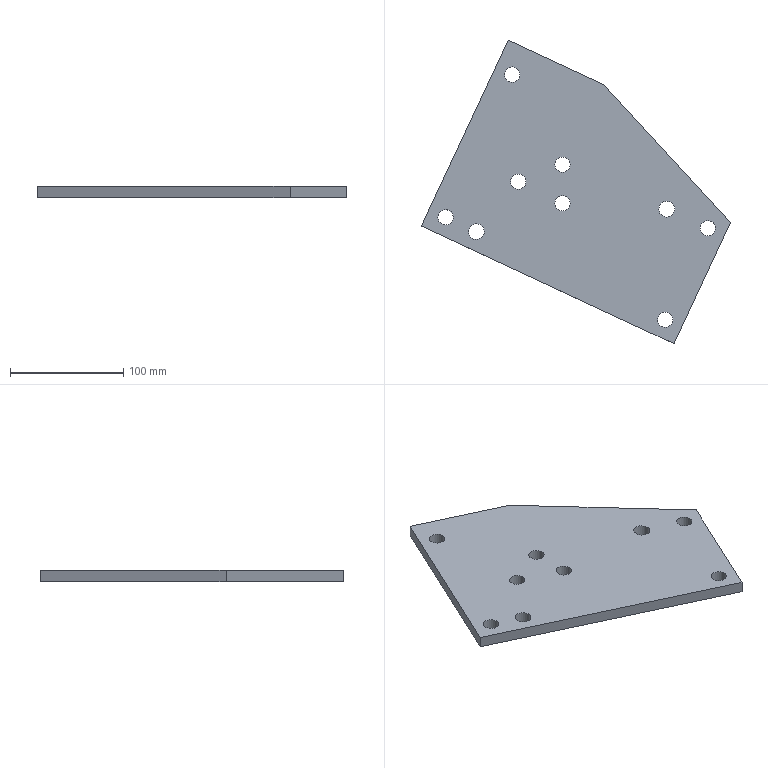Part | NX | features 6 2 | 1 solid | 16 faces | box 272.821 x 268.006 x 10 mm | volume 384202 mm3 | cylinder 9 | plane 7 | commonest cylinder face diameters 13.5 x7 14.001 x2
STEP:
#1=CARTESIAN_POINT('',(505.114,-156.901,101.));
#2=VERTEX_POINT('',#1);
#3=CARTESIAN_POINT('',(455.245,-263.846,101.));
#4=VERTEX_POINT('',#3);
#5=CARTESIAN_POINT('',(485.04,-199.951,101.));
#6=DIRECTION('',(-0.4226,-0.9063,0.));
#7=VECTOR('',#6,1000.);
#8=LINE('',#5,#7);
#9=EDGE_CURVE('',#2,#4,#8,.T.);
#10=ORIENTED_EDGE('',*,*,#9,.F.);
#11=CARTESIAN_POINT('',(393.754,-35.46,101.));
#12=VERTEX_POINT('',#11);
#13=CARTESIAN_POINT('',(202.399,173.217,101.));
#14=DIRECTION('',(-0.6759,0.737,0.));
#15=VECTOR('',#14,1000.);
#16=LINE('',#13,#15);
#17=EDGE_CURVE('',#2,#12,#16,.T.);
#18=ORIENTED_EDGE('',*,*,#17,.T.);
#19=CARTESIAN_POINT('',(308.788,4.16,101.));
#20=VERTEX_POINT('',#19);
#21=CARTESIAN_POINT('',(415.732,-45.709,101.));
#22=DIRECTION('',(0.9063,-0.4226,0.));
#23=VECTOR('',#22,1000.);
#24=LINE('',#21,#23);
#25=EDGE_CURVE('',#20,#12,#24,.T.);
#26=ORIENTED_EDGE('',*,*,#25,.F.);
#27=CARTESIAN_POINT('',(232.294,-159.881,101.));
#28=VERTEX_POINT('',#27);
#29=CARTESIAN_POINT('',(262.088,-95.987,101.));
#30=DIRECTION('',(0.4226,0.9063,0.));
#31=VECTOR('',#30,1000.);
#32=LINE('',#29,#31);
#33=EDGE_CURVE('',#28,#20,#32,.T.);
#34=ORIENTED_EDGE('',*,*,#33,.F.);
#35=CARTESIAN_POINT('',(339.238,-209.75,101.));
#36=DIRECTION('',(-0.9063,0.4226,0.));
#37=VECTOR('',#36,1000.);
#38=LINE('',#35,#37);
#39=EDGE_CURVE('',#4,#28,#38,.T.);
#40=ORIENTED_EDGE('',*,*,#39,.F.);
#41=EDGE_LOOP('',(#10,#18,#26,#34,#40));
#42=FACE_BOUND('',#41,.T.);
#43=CARTESIAN_POINT('',(455.212,-147.975,101.));
#44=VERTEX_POINT('',#43);
#45=CARTESIAN_POINT('',(448.867,-145.017,101.));
#46=DIRECTION('',(0.,0.,-1.));
#47=DIRECTION('',(0.9063,-0.4226,0.));
#48=AXIS2_PLACEMENT_3D('',#45,#46,#47);
#49=CIRCLE('',#48,7.);
#50=EDGE_CURVE('',#44,#44,#49,.T.);
#51=ORIENTED_EDGE('',*,*,#50,.T.);
#52=EDGE_LOOP('',(#51));
#53=FACE_BOUND('',#52,.T.);
#54=CARTESIAN_POINT('',(318.418,-29.018,101.));
#55=VERTEX_POINT('',#54);
#56=CARTESIAN_POINT('',(312.3,-26.166,101.));
#57=DIRECTION('',(0.,0.,-1.));
#58=DIRECTION('',(0.9063,-0.4226,0.));
#59=AXIS2_PLACEMENT_3D('',#56,#57,#58);
#60=CIRCLE('',#59,6.75);
#61=EDGE_CURVE('',#55,#55,#60,.T.);
#62=ORIENTED_EDGE('',*,*,#61,.T.);
#63=EDGE_LOOP('',(#62));
#64=FACE_BOUND('',#63,.T.);
#65=CARTESIAN_POINT('',(491.237,-164.774,101.));
#66=VERTEX_POINT('',#65);
#67=CARTESIAN_POINT('',(485.119,-161.921,101.));
#68=DIRECTION('',(0.,0.,-1.));
#69=DIRECTION('',(0.9063,-0.4226,0.));
#70=AXIS2_PLACEMENT_3D('',#67,#68,#69);
#71=CIRCLE('',#70,6.75);
#72=EDGE_CURVE('',#66,#66,#71,.T.);
#73=ORIENTED_EDGE('',*,*,#72,.T.);
#74=EDGE_LOOP('',(#73));
#75=FACE_BOUND('',#74,.T.);
#76=CARTESIAN_POINT('',(259.674,-154.995,101.));
#77=VERTEX_POINT('',#76);
#78=CARTESIAN_POINT('',(253.556,-152.142,101.));
#79=DIRECTION('',(0.,0.,-1.));
#80=DIRECTION('',(0.9063,-0.4226,0.));
#81=AXIS2_PLACEMENT_3D('',#78,#79,#80);
#82=CIRCLE('',#81,6.75);
#83=EDGE_CURVE('',#77,#77,#82,.T.);
#84=ORIENTED_EDGE('',*,*,#83,.T.);
#85=EDGE_LOOP('',(#84));
#86=FACE_BOUND('',#85,.T.);
#87=CARTESIAN_POINT('',(453.624,-245.435,101.));
#88=VERTEX_POINT('',#87);
#89=CARTESIAN_POINT('',(447.506,-242.583,101.));
#90=DIRECTION('',(0.,0.,-1.));
#91=DIRECTION('',(0.9063,-0.4226,0.));
#92=AXIS2_PLACEMENT_3D('',#89,#90,#91);
#93=CIRCLE('',#92,6.75);
#94=EDGE_CURVE('',#88,#88,#93,.T.);
#95=ORIENTED_EDGE('',*,*,#94,.T.);
#96=EDGE_LOOP('',(#95));
#97=FACE_BOUND('',#96,.T.);
#98=CARTESIAN_POINT('',(287.09,-167.779,101.));
#99=VERTEX_POINT('',#98);
#100=CARTESIAN_POINT('',(280.746,-164.821,101.));
#101=DIRECTION('',(0.,0.,-1.));
#102=DIRECTION('',(0.9063,-0.4226,0.));
#103=AXIS2_PLACEMENT_3D('',#100,#101,#102);
#104=CIRCLE('',#103,7.);
#105=EDGE_CURVE('',#99,#99,#104,.T.);
#106=ORIENTED_EDGE('',*,*,#105,.T.);
#107=EDGE_LOOP('',(#106));
#108=FACE_BOUND('',#107,.T.);
#109=CARTESIAN_POINT('',(363.523,-105.747,101.));
#110=VERTEX_POINT('',#109);
#111=CARTESIAN_POINT('',(356.773,-105.747,101.));
#112=DIRECTION('',(0.,0.,1.));
#113=DIRECTION('',(1.,0.,0.));
#114=AXIS2_PLACEMENT_3D('',#111,#112,#113);
#115=CIRCLE('',#114,6.75);
#116=EDGE_CURVE('',#110,#110,#115,.T.);
#117=ORIENTED_EDGE('',*,*,#116,.F.);
#118=EDGE_LOOP('',(#117));
#119=FACE_BOUND('',#118,.T.);
#120=CARTESIAN_POINT('',(363.523,-139.747,101.));
#121=VERTEX_POINT('',#120);
#122=CARTESIAN_POINT('',(356.773,-139.747,101.));
#123=DIRECTION('',(0.,0.,1.));
#124=DIRECTION('',(1.,0.,0.));
#125=AXIS2_PLACEMENT_3D('',#122,#123,#124);
#126=CIRCLE('',#125,6.75);
#127=EDGE_CURVE('',#121,#121,#126,.T.);
#128=ORIENTED_EDGE('',*,*,#127,.F.);
#129=EDGE_LOOP('',(#128));
#130=FACE_BOUND('',#129,.T.);
#131=CARTESIAN_POINT('',(324.523,-120.747,101.));
#132=VERTEX_POINT('',#131);
#133=CARTESIAN_POINT('',(317.773,-120.747,101.));
#134=DIRECTION('',(0.,0.,1.));
#135=DIRECTION('',(1.,0.,0.));
#136=AXIS2_PLACEMENT_3D('',#133,#134,#135);
#137=CIRCLE('',#136,6.75);
#138=EDGE_CURVE('',#132,#132,#137,.T.);
#139=ORIENTED_EDGE('',*,*,#138,.F.);
#140=EDGE_LOOP('',(#139));
#141=FACE_BOUND('',#140,.T.);
#142=CARTESIAN_POINT('',(239.919,207.622,101.));
#143=DIRECTION('',(0.,0.,1.));
#144=DIRECTION('',(-0.9063,0.4226,0.));
#145=AXIS2_PLACEMENT_3D('',#142,#143,#144);
#146=PLANE('',#145);
#147=ADVANCED_FACE('',(#42,#53,#64,#75,#86,#97,#108,#119,#130,#141),#146,.T.);
#148=CARTESIAN_POINT('',(393.754,-35.46,91.));
#149=VERTEX_POINT('',#148);
#150=CARTESIAN_POINT('',(308.788,4.16,91.));
#151=VERTEX_POINT('',#150);
#152=CARTESIAN_POINT('',(415.732,-45.709,91.));
#153=DIRECTION('',(-0.9063,0.4226,0.));
#154=VECTOR('',#153,1000.);
#155=LINE('',#152,#154);
#156=EDGE_CURVE('',#149,#151,#155,.T.);
#157=ORIENTED_EDGE('',*,*,#156,.F.);
#158=CARTESIAN_POINT('',(505.114,-156.901,91.));
#159=VERTEX_POINT('',#158);
#160=CARTESIAN_POINT('',(437.453,-83.115,91.));
#161=DIRECTION('',(0.6759,-0.737,0.));
#162=VECTOR('',#161,1000.);
#163=LINE('',#160,#162);
#164=EDGE_CURVE('',#149,#159,#163,.T.);
#165=ORIENTED_EDGE('',*,*,#164,.T.);
#166=CARTESIAN_POINT('',(455.245,-263.846,91.));
#167=VERTEX_POINT('',#166);
#168=CARTESIAN_POINT('',(485.04,-199.951,91.));
#169=DIRECTION('',(0.4226,0.9063,0.));
#170=VECTOR('',#169,1000.);
#171=LINE('',#168,#170);
#172=EDGE_CURVE('',#167,#159,#171,.T.);
#173=ORIENTED_EDGE('',*,*,#172,.F.);
#174=CARTESIAN_POINT('',(232.294,-159.881,91.));
#175=VERTEX_POINT('',#174);
#176=CARTESIAN_POINT('',(339.238,-209.75,91.));
#177=DIRECTION('',(0.9063,-0.4226,0.));
#178=VECTOR('',#177,1000.);
#179=LINE('',#176,#178);
#180=EDGE_CURVE('',#175,#167,#179,.T.);
#181=ORIENTED_EDGE('',*,*,#180,.F.);
#182=CARTESIAN_POINT('',(262.088,-95.987,91.));
#183=DIRECTION('',(-0.4226,-0.9063,0.));
#184=VECTOR('',#183,1000.);
#185=LINE('',#182,#184);
#186=EDGE_CURVE('',#151,#175,#185,.T.);
#187=ORIENTED_EDGE('',*,*,#186,.F.);
#188=EDGE_LOOP('',(#157,#165,#173,#181,#187));
#189=FACE_BOUND('',#188,.T.);
#190=CARTESIAN_POINT('',(455.212,-147.975,91.));
#191=VERTEX_POINT('',#190);
#192=CARTESIAN_POINT('',(448.867,-145.017,91.));
#193=DIRECTION('',(0.,0.,1.));
#194=DIRECTION('',(0.9063,-0.4226,0.));
#195=AXIS2_PLACEMENT_3D('',#192,#193,#194);
#196=CIRCLE('',#195,7.);
#197=EDGE_CURVE('',#191,#191,#196,.T.);
#198=ORIENTED_EDGE('',*,*,#197,.T.);
#199=EDGE_LOOP('',(#198));
#200=FACE_BOUND('',#199,.T.);
#201=CARTESIAN_POINT('',(318.418,-29.018,91.));
#202=VERTEX_POINT('',#201);
#203=CARTESIAN_POINT('',(312.3,-26.166,91.));
#204=DIRECTION('',(0.,0.,1.));
#205=DIRECTION('',(0.9063,-0.4226,0.));
#206=AXIS2_PLACEMENT_3D('',#203,#204,#205);
#207=CIRCLE('',#206,6.75);
#208=EDGE_CURVE('',#202,#202,#207,.T.);
#209=ORIENTED_EDGE('',*,*,#208,.T.);
#210=EDGE_LOOP('',(#209));
#211=FACE_BOUND('',#210,.T.);
#212=CARTESIAN_POINT('',(491.237,-164.774,91.));
#213=VERTEX_POINT('',#212);
#214=CARTESIAN_POINT('',(485.119,-161.921,91.));
#215=DIRECTION('',(0.,0.,1.));
#216=DIRECTION('',(0.9063,-0.4226,0.));
#217=AXIS2_PLACEMENT_3D('',#214,#215,#216);
#218=CIRCLE('',#217,6.75);
#219=EDGE_CURVE('',#213,#213,#218,.T.);
#220=ORIENTED_EDGE('',*,*,#219,.T.);
#221=EDGE_LOOP('',(#220));
#222=FACE_BOUND('',#221,.T.);
#223=CARTESIAN_POINT('',(259.674,-154.995,91.));
#224=VERTEX_POINT('',#223);
#225=CARTESIAN_POINT('',(253.556,-152.142,91.));
#226=DIRECTION('',(0.,0.,1.));
#227=DIRECTION('',(0.9063,-0.4226,0.));
#228=AXIS2_PLACEMENT_3D('',#225,#226,#227);
#229=CIRCLE('',#228,6.75);
#230=EDGE_CURVE('',#224,#224,#229,.T.);
#231=ORIENTED_EDGE('',*,*,#230,.T.);
#232=EDGE_LOOP('',(#231));
#233=FACE_BOUND('',#232,.T.);
#234=CARTESIAN_POINT('',(453.624,-245.435,91.));
#235=VERTEX_POINT('',#234);
#236=CARTESIAN_POINT('',(447.506,-242.583,91.));
#237=DIRECTION('',(0.,0.,1.));
#238=DIRECTION('',(0.9063,-0.4226,0.));
#239=AXIS2_PLACEMENT_3D('',#236,#237,#238);
#240=CIRCLE('',#239,6.75);
#241=EDGE_CURVE('',#235,#235,#240,.T.);
#242=ORIENTED_EDGE('',*,*,#241,.T.);
#243=EDGE_LOOP('',(#242));
#244=FACE_BOUND('',#243,.T.);
#245=CARTESIAN_POINT('',(287.09,-167.779,91.));
#246=VERTEX_POINT('',#245);
#247=CARTESIAN_POINT('',(280.746,-164.821,91.));
#248=DIRECTION('',(0.,0.,1.));
#249=DIRECTION('',(0.9063,-0.4226,0.));
#250=AXIS2_PLACEMENT_3D('',#247,#248,#249);
#251=CIRCLE('',#250,7.);
#252=EDGE_CURVE('',#246,#246,#251,.T.);
#253=ORIENTED_EDGE('',*,*,#252,.T.);
#254=EDGE_LOOP('',(#253));
#255=FACE_BOUND('',#254,.T.);
#256=CARTESIAN_POINT('',(350.023,-105.747,91.));
#257=VERTEX_POINT('',#256);
#258=CARTESIAN_POINT('',(356.773,-105.747,91.));
#259=DIRECTION('',(0.,0.,1.));
#260=DIRECTION('',(-1.,0.,0.));
#261=AXIS2_PLACEMENT_3D('',#258,#259,#260);
#262=CIRCLE('',#261,6.75);
#263=EDGE_CURVE('',#257,#257,#262,.T.);
#264=ORIENTED_EDGE('',*,*,#263,.T.);
#265=EDGE_LOOP('',(#264));
#266=FACE_BOUND('',#265,.T.);
#267=CARTESIAN_POINT('',(350.023,-139.747,91.));
#268=VERTEX_POINT('',#267);
#269=CARTESIAN_POINT('',(356.773,-139.747,91.));
#270=DIRECTION('',(0.,0.,1.));
#271=DIRECTION('',(-1.,0.,0.));
#272=AXIS2_PLACEMENT_3D('',#269,#270,#271);
#273=CIRCLE('',#272,6.75);
#274=EDGE_CURVE('',#268,#268,#273,.T.);
#275=ORIENTED_EDGE('',*,*,#274,.T.);
#276=EDGE_LOOP('',(#275));
#277=FACE_BOUND('',#276,.T.);
#278=CARTESIAN_POINT('',(311.023,-120.747,91.));
#279=VERTEX_POINT('',#278);
#280=CARTESIAN_POINT('',(317.773,-120.747,91.));
#281=DIRECTION('',(0.,0.,-1.));
#282=DIRECTION('',(-1.,0.,0.));
#283=AXIS2_PLACEMENT_3D('',#280,#281,#282);
#284=CIRCLE('',#283,6.75);
#285=EDGE_CURVE('',#279,#279,#284,.T.);
#286=ORIENTED_EDGE('',*,*,#285,.F.);
#287=EDGE_LOOP('',(#286));
#288=FACE_BOUND('',#287,.T.);
#289=CARTESIAN_POINT('',(369.033,-145.856,91.));
#290=DIRECTION('',(0.,0.,-1.));
#291=DIRECTION('',(0.9063,-0.4226,0.));
#292=AXIS2_PLACEMENT_3D('',#289,#290,#291);
#293=PLANE('',#292);
#294=ADVANCED_FACE('',(#189,#200,#211,#222,#233,#244,#255,#266,#277,#288),#293,.T.);
#295=ORIENTED_EDGE('',*,*,#25,.T.);
#296=CARTESIAN_POINT('',(393.754,-35.46,91.));
#297=DIRECTION('',(0.,0.,-1.));
#298=VECTOR('',#297,1000.);
#299=LINE('',#296,#298);
#300=EDGE_CURVE('',#12,#149,#299,.T.);
#301=ORIENTED_EDGE('',*,*,#300,.T.);
#302=ORIENTED_EDGE('',*,*,#156,.T.);
#303=CARTESIAN_POINT('',(308.788,4.16,91.));
#304=DIRECTION('',(0.,0.,1.));
#305=VECTOR('',#304,1000.);
#306=LINE('',#303,#305);
#307=EDGE_CURVE('',#151,#20,#306,.T.);
#308=ORIENTED_EDGE('',*,*,#307,.T.);
#309=EDGE_LOOP('',(#295,#301,#302,#308));
#310=FACE_BOUND('',#309,.T.);
#311=CARTESIAN_POINT('',(415.732,-45.709,91.));
#312=DIRECTION('',(0.4226,0.9063,0.));
#313=DIRECTION('',(0.,0.,-1.));
#314=AXIS2_PLACEMENT_3D('',#311,#312,#313);
#315=PLANE('',#314);
#316=ADVANCED_FACE('',(#310),#315,.T.);
#317=CARTESIAN_POINT('',(455.245,-263.846,91.));
#318=DIRECTION('',(0.,0.,1.));
#319=VECTOR('',#318,1000.);
#320=LINE('',#317,#319);
#321=EDGE_CURVE('',#167,#4,#320,.T.);
#322=ORIENTED_EDGE('',*,*,#321,.T.);
#323=ORIENTED_EDGE('',*,*,#39,.T.);
#324=CARTESIAN_POINT('',(232.294,-159.881,91.));
#325=DIRECTION('',(0.,0.,1.));
#326=VECTOR('',#325,1000.);
#327=LINE('',#324,#326);
#328=EDGE_CURVE('',#175,#28,#327,.T.);
#329=ORIENTED_EDGE('',*,*,#328,.F.);
#330=ORIENTED_EDGE('',*,*,#180,.T.);
#331=EDGE_LOOP('',(#322,#323,#329,#330));
#332=FACE_BOUND('',#331,.T.);
#333=CARTESIAN_POINT('',(339.238,-209.75,91.));
#334=DIRECTION('',(-0.4226,-0.9063,0.));
#335=DIRECTION('',(0.,0.,1.));
#336=AXIS2_PLACEMENT_3D('',#333,#334,#335);
#337=PLANE('',#336);
#338=ADVANCED_FACE('',(#332),#337,.T.);
#339=ORIENTED_EDGE('',*,*,#328,.T.);
#340=ORIENTED_EDGE('',*,*,#33,.T.);
#341=ORIENTED_EDGE('',*,*,#307,.F.);
#342=ORIENTED_EDGE('',*,*,#186,.T.);
#343=EDGE_LOOP('',(#339,#340,#341,#342));
#344=FACE_BOUND('',#343,.T.);
#345=CARTESIAN_POINT('',(262.088,-95.987,91.));
#346=DIRECTION('',(-0.9063,0.4226,0.));
#347=DIRECTION('',(0.,0.,-1.));
#348=AXIS2_PLACEMENT_3D('',#345,#346,#347);
#349=PLANE('',#348);
#350=ADVANCED_FACE('',(#344),#349,.T.);
#351=ORIENTED_EDGE('',*,*,#172,.T.);
#352=CARTESIAN_POINT('',(505.114,-156.901,91.));
#353=DIRECTION('',(0.,0.,1.));
#354=VECTOR('',#353,1000.);
#355=LINE('',#352,#354);
#356=EDGE_CURVE('',#159,#2,#355,.T.);
#357=ORIENTED_EDGE('',*,*,#356,.T.);
#358=ORIENTED_EDGE('',*,*,#9,.T.);
#359=ORIENTED_EDGE('',*,*,#321,.F.);
#360=EDGE_LOOP('',(#351,#357,#358,#359));
#361=FACE_BOUND('',#360,.T.);
#362=CARTESIAN_POINT('',(485.04,-199.951,91.));
#363=DIRECTION('',(0.9063,-0.4226,0.));
#364=DIRECTION('',(0.,0.,1.));
#365=AXIS2_PLACEMENT_3D('',#362,#363,#364);
#366=PLANE('',#365);
#367=ADVANCED_FACE('',(#361),#366,.T.);
#368=ORIENTED_EDGE('',*,*,#83,.F.);
#369=EDGE_LOOP('',(#368));
#370=FACE_BOUND('',#369,.T.);
#371=ORIENTED_EDGE('',*,*,#230,.F.);
#372=EDGE_LOOP('',(#371));
#373=FACE_BOUND('',#372,.T.);
#374=CARTESIAN_POINT('',(253.556,-152.142,91.));
#375=DIRECTION('',(0.,0.,1.));
#376=DIRECTION('',(-0.9063,0.4226,0.));
#377=AXIS2_PLACEMENT_3D('',#374,#375,#376);
#378=CYLINDRICAL_SURFACE('',#377,6.75);
#379=ADVANCED_FACE('',(#370,#373),#378,.F.);
#380=ORIENTED_EDGE('',*,*,#72,.F.);
#381=EDGE_LOOP('',(#380));
#382=FACE_BOUND('',#381,.T.);
#383=ORIENTED_EDGE('',*,*,#219,.F.);
#384=EDGE_LOOP('',(#383));
#385=FACE_BOUND('',#384,.T.);
#386=CARTESIAN_POINT('',(485.119,-161.921,91.));
#387=DIRECTION('',(0.,0.,1.));
#388=DIRECTION('',(-0.9063,0.4226,0.));
#389=AXIS2_PLACEMENT_3D('',#386,#387,#388);
#390=CYLINDRICAL_SURFACE('',#389,6.75);
#391=ADVANCED_FACE('',(#382,#385),#390,.F.);
#392=ORIENTED_EDGE('',*,*,#94,.F.);
#393=EDGE_LOOP('',(#392));
#394=FACE_BOUND('',#393,.T.);
#395=ORIENTED_EDGE('',*,*,#241,.F.);
#396=EDGE_LOOP('',(#395));
#397=FACE_BOUND('',#396,.T.);
#398=CARTESIAN_POINT('',(447.506,-242.583,91.));
#399=DIRECTION('',(0.,0.,1.));
#400=DIRECTION('',(-0.9063,0.4226,0.));
#401=AXIS2_PLACEMENT_3D('',#398,#399,#400);
#402=CYLINDRICAL_SURFACE('',#401,6.75);
#403=ADVANCED_FACE('',(#394,#397),#402,.F.);
#404=ORIENTED_EDGE('',*,*,#61,.F.);
#405=EDGE_LOOP('',(#404));
#406=FACE_BOUND('',#405,.T.);
#407=ORIENTED_EDGE('',*,*,#208,.F.);
#408=EDGE_LOOP('',(#407));
#409=FACE_BOUND('',#408,.T.);
#410=CARTESIAN_POINT('',(312.3,-26.166,91.));
#411=DIRECTION('',(0.,0.,1.));
#412=DIRECTION('',(-0.9063,0.4226,0.));
#413=AXIS2_PLACEMENT_3D('',#410,#411,#412);
#414=CYLINDRICAL_SURFACE('',#413,6.75);
#415=ADVANCED_FACE('',(#406,#409),#414,.F.);
#416=ORIENTED_EDGE('',*,*,#105,.F.);
#417=EDGE_LOOP('',(#416));
#418=FACE_BOUND('',#417,.T.);
#419=ORIENTED_EDGE('',*,*,#252,.F.);
#420=EDGE_LOOP('',(#419));
#421=FACE_BOUND('',#420,.T.);
#422=CARTESIAN_POINT('',(280.746,-164.821,91.));
#423=DIRECTION('',(0.,0.,1.));
#424=DIRECTION('',(-0.9063,0.4226,0.));
#425=AXIS2_PLACEMENT_3D('',#422,#423,#424);
#426=CYLINDRICAL_SURFACE('',#425,7.);
#427=ADVANCED_FACE('',(#418,#421),#426,.F.);
#428=ORIENTED_EDGE('',*,*,#50,.F.);
#429=EDGE_LOOP('',(#428));
#430=FACE_BOUND('',#429,.T.);
#431=ORIENTED_EDGE('',*,*,#197,.F.);
#432=EDGE_LOOP('',(#431));
#433=FACE_BOUND('',#432,.T.);
#434=CARTESIAN_POINT('',(448.867,-145.017,91.));
#435=DIRECTION('',(0.,0.,1.));
#436=DIRECTION('',(-0.9063,0.4226,0.));
#437=AXIS2_PLACEMENT_3D('',#434,#435,#436);
#438=CYLINDRICAL_SURFACE('',#437,7.);
#439=ADVANCED_FACE('',(#430,#433),#438,.F.);
#440=ORIENTED_EDGE('',*,*,#116,.T.);
#441=EDGE_LOOP('',(#440));
#442=FACE_BOUND('',#441,.T.);
#443=ORIENTED_EDGE('',*,*,#263,.F.);
#444=EDGE_LOOP('',(#443));
#445=FACE_BOUND('',#444,.T.);
#446=CARTESIAN_POINT('',(356.773,-105.747,-61.));
#447=DIRECTION('',(0.,0.,1.));
#448=DIRECTION('',(-1.,0.,0.));
#449=AXIS2_PLACEMENT_3D('',#446,#447,#448);
#450=CYLINDRICAL_SURFACE('',#449,6.75);
#451=ADVANCED_FACE('',(#442,#445),#450,.F.);
#452=ORIENTED_EDGE('',*,*,#127,.T.);
#453=EDGE_LOOP('',(#452));
#454=FACE_BOUND('',#453,.T.);
#455=ORIENTED_EDGE('',*,*,#274,.F.);
#456=EDGE_LOOP('',(#455));
#457=FACE_BOUND('',#456,.T.);
#458=CARTESIAN_POINT('',(356.773,-139.747,-61.));
#459=DIRECTION('',(0.,0.,1.));
#460=DIRECTION('',(-1.,0.,0.));
#461=AXIS2_PLACEMENT_3D('',#458,#459,#460);
#462=CYLINDRICAL_SURFACE('',#461,6.75);
#463=ADVANCED_FACE('',(#454,#457),#462,.F.);
#464=ORIENTED_EDGE('',*,*,#138,.T.);
#465=EDGE_LOOP('',(#464));
#466=FACE_BOUND('',#465,.T.);
#467=ORIENTED_EDGE('',*,*,#285,.T.);
#468=EDGE_LOOP('',(#467));
#469=FACE_BOUND('',#468,.T.);
#470=CARTESIAN_POINT('',(317.773,-120.747,-61.));
#471=DIRECTION('',(0.,0.,1.));
#472=DIRECTION('',(-1.,0.,0.));
#473=AXIS2_PLACEMENT_3D('',#470,#471,#472);
#474=CYLINDRICAL_SURFACE('',#473,6.75);
#475=ADVANCED_FACE('',(#466,#469),#474,.F.);
#476=ORIENTED_EDGE('',*,*,#164,.F.);
#477=ORIENTED_EDGE('',*,*,#300,.F.);
#478=ORIENTED_EDGE('',*,*,#17,.F.);
#479=ORIENTED_EDGE('',*,*,#356,.F.);
#480=EDGE_LOOP('',(#476,#477,#478,#479));
#481=FACE_BOUND('',#480,.T.);
#482=CARTESIAN_POINT('',(505.114,-156.901,91.));
#483=DIRECTION('',(-0.737,-0.6759,0.));
#484=DIRECTION('',(0.,0.,-1.));
#485=AXIS2_PLACEMENT_3D('',#482,#483,#484);
#486=PLANE('',#485);
#487=ADVANCED_FACE('',(#481),#486,.F.);
#488=CLOSED_SHELL('',(#147,#294,#316,#338,#350,#367,#379,#391,#403,#415,#427,#439,#451,#463,#475,#487));
#489=MANIFOLD_SOLID_BREP('',#488);
#490=(LENGTH_UNIT()NAMED_UNIT(*)SI_UNIT(.MILLI.,.METRE.));
#491=UNCERTAINTY_MEASURE_WITH_UNIT(LENGTH_MEASURE(0.00001),#490,'','');
#492=(NAMED_UNIT(*)PLANE_ANGLE_UNIT()SI_UNIT($,.RADIAN.));
#493=(NAMED_UNIT(*)SI_UNIT($,.STERADIAN.)SOLID_ANGLE_UNIT());
#494=(GEOMETRIC_REPRESENTATION_CONTEXT(3)GLOBAL_UNCERTAINTY_ASSIGNED_CONTEXT((#491))GLOBAL_UNIT_ASSIGNED_CONTEXT((#490,#492,#493))REPRESENTATION_CONTEXT('',''));
#495=ADVANCED_BREP_SHAPE_REPRESENTATION('',(#489),#494);